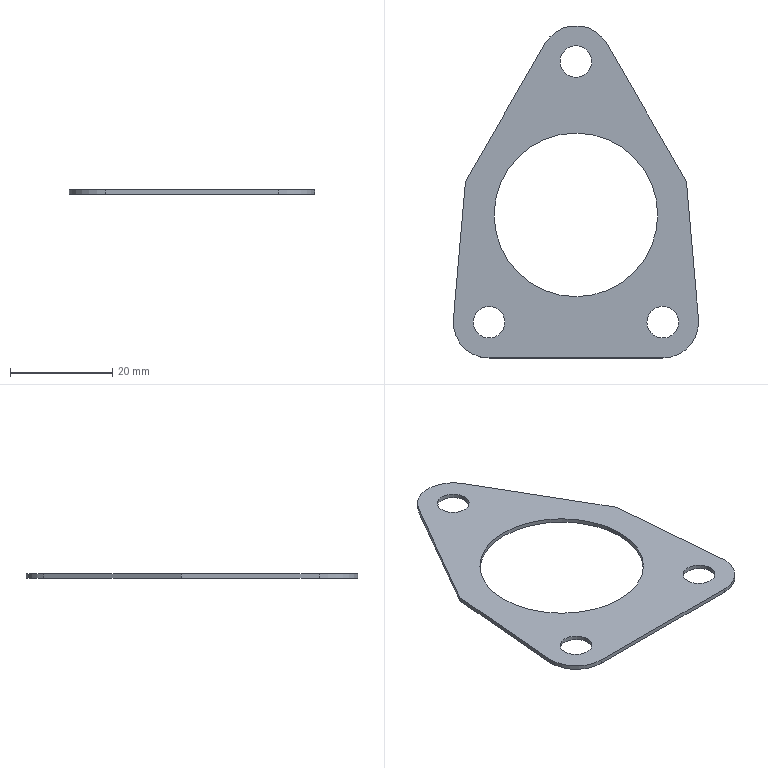Part | SolidWorks | features BaseBody 1 | 1 solid | 19 faces | box 48 x 65 x 0.8 mm | volume 1163 mm3 | cylinder 12 | plane 7 | commonest cylinder face diameters 6.2 x6 14 x4 32 x2
STEP:
#1=CARTESIAN_POINT('',(113.6,-21.,50.5));
#2=VERTEX_POINT('',#1);
#3=CARTESIAN_POINT('',(107.4,-21.,50.5));
#4=VERTEX_POINT('',#3);
#5=CARTESIAN_POINT('',(110.5,-21.,50.5));
#6=DIRECTION('',(0.,0.,-1.));
#7=DIRECTION('',(-1.,0.,0.));
#8=AXIS2_PLACEMENT_3D('',#5,#6,#7);
#9=CIRCLE('',#8,3.1);
#10=EDGE_CURVE('',#2,#4,#9,.T.);
#11=ORIENTED_EDGE('',*,*,#10,.T.);
#12=CARTESIAN_POINT('',(107.4,-21.,51.3));
#13=VERTEX_POINT('',#12);
#14=CARTESIAN_POINT('',(107.4,-21.,50.5));
#15=DIRECTION('',(0.,0.,1.));
#16=VECTOR('',#15,1000.);
#17=LINE('',#14,#16);
#18=EDGE_CURVE('',#4,#13,#17,.T.);
#19=ORIENTED_EDGE('',*,*,#18,.T.);
#20=CARTESIAN_POINT('',(113.6,-21.,51.3));
#21=VERTEX_POINT('',#20);
#22=CARTESIAN_POINT('',(110.5,-21.,51.3));
#23=DIRECTION('',(0.,0.,-1.));
#24=DIRECTION('',(-1.,0.,0.));
#25=AXIS2_PLACEMENT_3D('',#22,#23,#24);
#26=CIRCLE('',#25,3.1);
#27=EDGE_CURVE('',#21,#13,#26,.T.);
#28=ORIENTED_EDGE('',*,*,#27,.F.);
#29=CARTESIAN_POINT('',(113.6,-21.,50.5));
#30=DIRECTION('',(0.,0.,1.));
#31=VECTOR('',#30,1000.);
#32=LINE('',#29,#31);
#33=EDGE_CURVE('',#2,#21,#32,.T.);
#34=ORIENTED_EDGE('',*,*,#33,.F.);
#35=EDGE_LOOP('',(#11,#19,#28,#34));
#36=FACE_OUTER_BOUND('',#35,.T.);
#37=CARTESIAN_POINT('',(110.5,-21.,50.5));
#38=DIRECTION('',(0.,0.,1.));
#39=DIRECTION('',(1.,0.,0.));
#40=AXIS2_PLACEMENT_3D('',#37,#38,#39);
#41=CYLINDRICAL_SURFACE('',#40,3.1);
#42=ADVANCED_FACE('',(#36),#41,.F.);
#43=CARTESIAN_POINT('',(79.6,-21.,50.5));
#44=VERTEX_POINT('',#43);
#45=CARTESIAN_POINT('',(73.4,-21.,50.5));
#46=VERTEX_POINT('',#45);
#47=CARTESIAN_POINT('',(76.5,-21.,50.5));
#48=DIRECTION('',(0.,0.,-1.));
#49=DIRECTION('',(-1.,0.,0.));
#50=AXIS2_PLACEMENT_3D('',#47,#48,#49);
#51=CIRCLE('',#50,3.1);
#52=EDGE_CURVE('',#44,#46,#51,.T.);
#53=ORIENTED_EDGE('',*,*,#52,.T.);
#54=CARTESIAN_POINT('',(73.4,-21.,51.3));
#55=VERTEX_POINT('',#54);
#56=CARTESIAN_POINT('',(73.4,-21.,50.5));
#57=DIRECTION('',(0.,0.,1.));
#58=VECTOR('',#57,1000.);
#59=LINE('',#56,#58);
#60=EDGE_CURVE('',#46,#55,#59,.T.);
#61=ORIENTED_EDGE('',*,*,#60,.T.);
#62=CARTESIAN_POINT('',(79.6,-21.,51.3));
#63=VERTEX_POINT('',#62);
#64=CARTESIAN_POINT('',(76.5,-21.,51.3));
#65=DIRECTION('',(0.,0.,-1.));
#66=DIRECTION('',(-1.,0.,0.));
#67=AXIS2_PLACEMENT_3D('',#64,#65,#66);
#68=CIRCLE('',#67,3.1);
#69=EDGE_CURVE('',#63,#55,#68,.T.);
#70=ORIENTED_EDGE('',*,*,#69,.F.);
#71=CARTESIAN_POINT('',(79.6,-21.,50.5));
#72=DIRECTION('',(0.,0.,1.));
#73=VECTOR('',#72,1000.);
#74=LINE('',#71,#73);
#75=EDGE_CURVE('',#44,#63,#74,.T.);
#76=ORIENTED_EDGE('',*,*,#75,.F.);
#77=EDGE_LOOP('',(#53,#61,#70,#76));
#78=FACE_OUTER_BOUND('',#77,.T.);
#79=CARTESIAN_POINT('',(76.5,-21.,50.5));
#80=DIRECTION('',(0.,0.,1.));
#81=DIRECTION('',(1.,0.,0.));
#82=AXIS2_PLACEMENT_3D('',#79,#80,#81);
#83=CYLINDRICAL_SURFACE('',#82,3.1);
#84=ADVANCED_FACE('',(#78),#83,.F.);
#85=CARTESIAN_POINT('',(96.6,30.,50.5));
#86=VERTEX_POINT('',#85);
#87=CARTESIAN_POINT('',(90.4,30.,50.5));
#88=VERTEX_POINT('',#87);
#89=CARTESIAN_POINT('',(93.5,30.,50.5));
#90=DIRECTION('',(0.,0.,-1.));
#91=DIRECTION('',(-1.,0.,0.));
#92=AXIS2_PLACEMENT_3D('',#89,#90,#91);
#93=CIRCLE('',#92,3.1);
#94=EDGE_CURVE('',#86,#88,#93,.T.);
#95=ORIENTED_EDGE('',*,*,#94,.T.);
#96=CARTESIAN_POINT('',(90.4,30.,51.3));
#97=VERTEX_POINT('',#96);
#98=CARTESIAN_POINT('',(90.4,30.,50.5));
#99=DIRECTION('',(0.,0.,1.));
#100=VECTOR('',#99,1000.);
#101=LINE('',#98,#100);
#102=EDGE_CURVE('',#88,#97,#101,.T.);
#103=ORIENTED_EDGE('',*,*,#102,.T.);
#104=CARTESIAN_POINT('',(96.6,30.,51.3));
#105=VERTEX_POINT('',#104);
#106=CARTESIAN_POINT('',(93.5,30.,51.3));
#107=DIRECTION('',(0.,0.,-1.));
#108=DIRECTION('',(-1.,0.,0.));
#109=AXIS2_PLACEMENT_3D('',#106,#107,#108);
#110=CIRCLE('',#109,3.1);
#111=EDGE_CURVE('',#105,#97,#110,.T.);
#112=ORIENTED_EDGE('',*,*,#111,.F.);
#113=CARTESIAN_POINT('',(96.6,30.,50.5));
#114=DIRECTION('',(0.,0.,1.));
#115=VECTOR('',#114,1000.);
#116=LINE('',#113,#115);
#117=EDGE_CURVE('',#86,#105,#116,.T.);
#118=ORIENTED_EDGE('',*,*,#117,.F.);
#119=EDGE_LOOP('',(#95,#103,#112,#118));
#120=FACE_OUTER_BOUND('',#119,.T.);
#121=CARTESIAN_POINT('',(93.5,30.,50.5));
#122=DIRECTION('',(0.,0.,1.));
#123=DIRECTION('',(1.,0.,0.));
#124=AXIS2_PLACEMENT_3D('',#121,#122,#123);
#125=CYLINDRICAL_SURFACE('',#124,3.1);
#126=ADVANCED_FACE('',(#120),#125,.F.);
#127=CARTESIAN_POINT('',(109.5,0.,50.5));
#128=VERTEX_POINT('',#127);
#129=CARTESIAN_POINT('',(77.5,0.,50.5));
#130=VERTEX_POINT('',#129);
#131=CARTESIAN_POINT('',(93.5,0.,50.5));
#132=DIRECTION('',(0.,0.,-1.));
#133=DIRECTION('',(-1.,0.,0.));
#134=AXIS2_PLACEMENT_3D('',#131,#132,#133);
#135=CIRCLE('',#134,16.);
#136=EDGE_CURVE('',#128,#130,#135,.T.);
#137=ORIENTED_EDGE('',*,*,#136,.T.);
#138=CARTESIAN_POINT('',(77.5,0.,51.3));
#139=VERTEX_POINT('',#138);
#140=CARTESIAN_POINT('',(77.5,0.,50.5));
#141=DIRECTION('',(0.,0.,1.));
#142=VECTOR('',#141,1000.);
#143=LINE('',#140,#142);
#144=EDGE_CURVE('',#130,#139,#143,.T.);
#145=ORIENTED_EDGE('',*,*,#144,.T.);
#146=CARTESIAN_POINT('',(109.5,0.,51.3));
#147=VERTEX_POINT('',#146);
#148=CARTESIAN_POINT('',(93.5,0.,51.3));
#149=DIRECTION('',(0.,0.,-1.));
#150=DIRECTION('',(-1.,0.,0.));
#151=AXIS2_PLACEMENT_3D('',#148,#149,#150);
#152=CIRCLE('',#151,16.);
#153=EDGE_CURVE('',#147,#139,#152,.T.);
#154=ORIENTED_EDGE('',*,*,#153,.F.);
#155=CARTESIAN_POINT('',(109.5,0.,50.5));
#156=DIRECTION('',(0.,0.,1.));
#157=VECTOR('',#156,1000.);
#158=LINE('',#155,#157);
#159=EDGE_CURVE('',#128,#147,#158,.T.);
#160=ORIENTED_EDGE('',*,*,#159,.F.);
#161=EDGE_LOOP('',(#137,#145,#154,#160));
#162=FACE_OUTER_BOUND('',#161,.T.);
#163=CARTESIAN_POINT('',(93.5,0.,50.5));
#164=DIRECTION('',(0.,0.,1.));
#165=DIRECTION('',(1.,0.,0.));
#166=AXIS2_PLACEMENT_3D('',#163,#164,#165);
#167=CYLINDRICAL_SURFACE('',#166,16.);
#168=ADVANCED_FACE('',(#162),#167,.F.);
#169=CARTESIAN_POINT('',(117.5,-21.,50.5));
#170=VERTEX_POINT('',#169);
#171=CARTESIAN_POINT('',(110.5,-28.,50.5));
#172=VERTEX_POINT('',#171);
#173=CARTESIAN_POINT('',(110.5,-21.,50.5));
#174=DIRECTION('',(0.,0.,-1.));
#175=DIRECTION('',(-1.,0.,0.));
#176=AXIS2_PLACEMENT_3D('',#173,#174,#175);
#177=CIRCLE('',#176,7.);
#178=EDGE_CURVE('',#170,#172,#177,.T.);
#179=ORIENTED_EDGE('',*,*,#178,.F.);
#180=CARTESIAN_POINT('',(117.5,-21.,51.3));
#181=VERTEX_POINT('',#180);
#182=CARTESIAN_POINT('',(117.5,-21.,50.5));
#183=DIRECTION('',(0.,0.,1.));
#184=VECTOR('',#183,1000.);
#185=LINE('',#182,#184);
#186=EDGE_CURVE('',#170,#181,#185,.T.);
#187=ORIENTED_EDGE('',*,*,#186,.T.);
#188=CARTESIAN_POINT('',(110.5,-28.,51.3));
#189=VERTEX_POINT('',#188);
#190=CARTESIAN_POINT('',(110.5,-21.,51.3));
#191=DIRECTION('',(0.,0.,-1.));
#192=DIRECTION('',(-1.,0.,0.));
#193=AXIS2_PLACEMENT_3D('',#190,#191,#192);
#194=CIRCLE('',#193,7.);
#195=EDGE_CURVE('',#181,#189,#194,.T.);
#196=ORIENTED_EDGE('',*,*,#195,.T.);
#197=CARTESIAN_POINT('',(110.5,-28.,50.5));
#198=DIRECTION('',(0.,0.,1.));
#199=VECTOR('',#198,1000.);
#200=LINE('',#197,#199);
#201=EDGE_CURVE('',#172,#189,#200,.T.);
#202=ORIENTED_EDGE('',*,*,#201,.F.);
#203=EDGE_LOOP('',(#179,#187,#196,#202));
#204=FACE_OUTER_BOUND('',#203,.T.);
#205=CARTESIAN_POINT('',(110.5,-21.,50.5));
#206=DIRECTION('',(0.,0.,1.));
#207=DIRECTION('',(1.,0.,0.));
#208=AXIS2_PLACEMENT_3D('',#205,#206,#207);
#209=CYLINDRICAL_SURFACE('',#208,7.);
#210=ADVANCED_FACE('',(#204),#209,.T.);
#211=ORIENTED_EDGE('',*,*,#52,.F.);
#212=CARTESIAN_POINT('',(76.5,-21.,50.5));
#213=DIRECTION('',(0.,0.,-1.));
#214=DIRECTION('',(-1.,0.,0.));
#215=AXIS2_PLACEMENT_3D('',#212,#213,#214);
#216=CIRCLE('',#215,3.1);
#217=EDGE_CURVE('',#46,#44,#216,.T.);
#218=ORIENTED_EDGE('',*,*,#217,.F.);
#219=EDGE_LOOP('',(#211,#218));
#220=FACE_BOUND('',#219,.T.);
#221=ORIENTED_EDGE('',*,*,#136,.F.);
#222=CARTESIAN_POINT('',(93.5,0.,50.5));
#223=DIRECTION('',(0.,0.,-1.));
#224=DIRECTION('',(-1.,0.,0.));
#225=AXIS2_PLACEMENT_3D('',#222,#223,#224);
#226=CIRCLE('',#225,16.);
#227=EDGE_CURVE('',#130,#128,#226,.T.);
#228=ORIENTED_EDGE('',*,*,#227,.F.);
#229=EDGE_LOOP('',(#221,#228));
#230=FACE_BOUND('',#229,.T.);
#231=CARTESIAN_POINT('',(87.438,33.5,50.5));
#232=VERTEX_POINT('',#231);
#233=CARTESIAN_POINT('',(99.562,33.5,50.5));
#234=VERTEX_POINT('',#233);
#235=CARTESIAN_POINT('',(93.5,30.,50.5));
#236=DIRECTION('',(0.,0.,-1.));
#237=DIRECTION('',(-1.,0.,0.));
#238=AXIS2_PLACEMENT_3D('',#235,#236,#237);
#239=CIRCLE('',#238,7.);
#240=EDGE_CURVE('',#232,#234,#239,.T.);
#241=ORIENTED_EDGE('',*,*,#240,.T.);
#242=CARTESIAN_POINT('',(115.115,6.561,50.5));
#243=VERTEX_POINT('',#242);
#244=CARTESIAN_POINT('',(99.562,33.5,50.5));
#245=DIRECTION('',(0.5,-0.866,0.));
#246=VECTOR('',#245,1000.);
#247=LINE('',#244,#246);
#248=EDGE_CURVE('',#234,#243,#247,.T.);
#249=ORIENTED_EDGE('',*,*,#248,.T.);
#250=CARTESIAN_POINT('',(117.473,-20.39,50.5));
#251=VERTEX_POINT('',#250);
#252=CARTESIAN_POINT('',(117.473,-20.39,50.5));
#253=DIRECTION('',(0.08716,-0.9962,0.));
#254=VECTOR('',#253,1000.);
#255=LINE('',#252,#254);
#256=EDGE_CURVE('',#243,#251,#255,.T.);
#257=ORIENTED_EDGE('',*,*,#256,.T.);
#258=CARTESIAN_POINT('',(110.5,-21.,50.5));
#259=DIRECTION('',(0.,0.,-1.));
#260=DIRECTION('',(-1.,0.,0.));
#261=AXIS2_PLACEMENT_3D('',#258,#259,#260);
#262=CIRCLE('',#261,7.);
#263=EDGE_CURVE('',#251,#170,#262,.T.);
#264=ORIENTED_EDGE('',*,*,#263,.T.);
#265=ORIENTED_EDGE('',*,*,#178,.T.);
#266=CARTESIAN_POINT('',(76.5,-28.,50.5));
#267=VERTEX_POINT('',#266);
#268=CARTESIAN_POINT('',(110.5,-28.,50.5));
#269=DIRECTION('',(-1.,0.,0.));
#270=VECTOR('',#269,1000.);
#271=LINE('',#268,#270);
#272=EDGE_CURVE('',#172,#267,#271,.T.);
#273=ORIENTED_EDGE('',*,*,#272,.T.);
#274=CARTESIAN_POINT('',(69.527,-20.39,50.5));
#275=VERTEX_POINT('',#274);
#276=CARTESIAN_POINT('',(76.5,-21.,50.5));
#277=DIRECTION('',(0.,0.,-1.));
#278=DIRECTION('',(-1.,0.,0.));
#279=AXIS2_PLACEMENT_3D('',#276,#277,#278);
#280=CIRCLE('',#279,7.);
#281=EDGE_CURVE('',#267,#275,#280,.T.);
#282=ORIENTED_EDGE('',*,*,#281,.T.);
#283=CARTESIAN_POINT('',(71.885,6.561,50.5));
#284=VERTEX_POINT('',#283);
#285=CARTESIAN_POINT('',(69.527,-20.39,50.5));
#286=DIRECTION('',(0.08716,0.9962,0.));
#287=VECTOR('',#286,1000.);
#288=LINE('',#285,#287);
#289=EDGE_CURVE('',#275,#284,#288,.T.);
#290=ORIENTED_EDGE('',*,*,#289,.T.);
#291=CARTESIAN_POINT('',(87.438,33.5,50.5));
#292=DIRECTION('',(0.5,0.866,0.));
#293=VECTOR('',#292,1000.);
#294=LINE('',#291,#293);
#295=EDGE_CURVE('',#284,#232,#294,.T.);
#296=ORIENTED_EDGE('',*,*,#295,.T.);
#297=EDGE_LOOP('',(#241,#249,#257,#264,#265,#273,#282,#290,#296));
#298=FACE_OUTER_BOUND('',#297,.T.);
#299=ORIENTED_EDGE('',*,*,#94,.F.);
#300=CARTESIAN_POINT('',(93.5,30.,50.5));
#301=DIRECTION('',(0.,0.,-1.));
#302=DIRECTION('',(-1.,0.,0.));
#303=AXIS2_PLACEMENT_3D('',#300,#301,#302);
#304=CIRCLE('',#303,3.1);
#305=EDGE_CURVE('',#88,#86,#304,.T.);
#306=ORIENTED_EDGE('',*,*,#305,.F.);
#307=EDGE_LOOP('',(#299,#306));
#308=FACE_BOUND('',#307,.T.);
#309=ORIENTED_EDGE('',*,*,#10,.F.);
#310=CARTESIAN_POINT('',(110.5,-21.,50.5));
#311=DIRECTION('',(0.,0.,-1.));
#312=DIRECTION('',(-1.,0.,0.));
#313=AXIS2_PLACEMENT_3D('',#310,#311,#312);
#314=CIRCLE('',#313,3.1);
#315=EDGE_CURVE('',#4,#2,#314,.T.);
#316=ORIENTED_EDGE('',*,*,#315,.F.);
#317=EDGE_LOOP('',(#309,#316));
#318=FACE_BOUND('',#317,.T.);
#319=CARTESIAN_POINT('',(93.5,30.,50.5));
#320=DIRECTION('',(0.,0.,-1.));
#321=DIRECTION('',(-1.,0.,0.));
#322=AXIS2_PLACEMENT_3D('',#319,#320,#321);
#323=PLANE('',#322);
#324=ADVANCED_FACE('',(#220,#230,#298,#308,#318),#323,.T.);
#325=ORIENTED_EDGE('',*,*,#69,.T.);
#326=CARTESIAN_POINT('',(76.5,-21.,51.3));
#327=DIRECTION('',(0.,0.,-1.));
#328=DIRECTION('',(-1.,0.,0.));
#329=AXIS2_PLACEMENT_3D('',#326,#327,#328);
#330=CIRCLE('',#329,3.1);
#331=EDGE_CURVE('',#55,#63,#330,.T.);
#332=ORIENTED_EDGE('',*,*,#331,.T.);
#333=EDGE_LOOP('',(#325,#332));
#334=FACE_BOUND('',#333,.T.);
#335=ORIENTED_EDGE('',*,*,#153,.T.);
#336=CARTESIAN_POINT('',(93.5,0.,51.3));
#337=DIRECTION('',(0.,0.,-1.));
#338=DIRECTION('',(-1.,0.,0.));
#339=AXIS2_PLACEMENT_3D('',#336,#337,#338);
#340=CIRCLE('',#339,16.);
#341=EDGE_CURVE('',#139,#147,#340,.T.);
#342=ORIENTED_EDGE('',*,*,#341,.T.);
#343=EDGE_LOOP('',(#335,#342));
#344=FACE_BOUND('',#343,.T.);
#345=CARTESIAN_POINT('',(87.438,33.5,51.3));
#346=VERTEX_POINT('',#345);
#347=CARTESIAN_POINT('',(99.562,33.5,51.3));
#348=VERTEX_POINT('',#347);
#349=CARTESIAN_POINT('',(93.5,30.,51.3));
#350=DIRECTION('',(0.,0.,-1.));
#351=DIRECTION('',(-1.,0.,0.));
#352=AXIS2_PLACEMENT_3D('',#349,#350,#351);
#353=CIRCLE('',#352,7.);
#354=EDGE_CURVE('',#346,#348,#353,.T.);
#355=ORIENTED_EDGE('',*,*,#354,.F.);
#356=CARTESIAN_POINT('',(71.885,6.561,51.3));
#357=VERTEX_POINT('',#356);
#358=CARTESIAN_POINT('',(87.438,33.5,51.3));
#359=DIRECTION('',(0.5,0.866,0.));
#360=VECTOR('',#359,1000.);
#361=LINE('',#358,#360);
#362=EDGE_CURVE('',#357,#346,#361,.T.);
#363=ORIENTED_EDGE('',*,*,#362,.F.);
#364=CARTESIAN_POINT('',(69.527,-20.39,51.3));
#365=VERTEX_POINT('',#364);
#366=CARTESIAN_POINT('',(69.527,-20.39,51.3));
#367=DIRECTION('',(0.08716,0.9962,0.));
#368=VECTOR('',#367,1000.);
#369=LINE('',#366,#368);
#370=EDGE_CURVE('',#365,#357,#369,.T.);
#371=ORIENTED_EDGE('',*,*,#370,.F.);
#372=CARTESIAN_POINT('',(76.5,-28.,51.3));
#373=VERTEX_POINT('',#372);
#374=CARTESIAN_POINT('',(76.5,-21.,51.3));
#375=DIRECTION('',(0.,0.,-1.));
#376=DIRECTION('',(-1.,0.,0.));
#377=AXIS2_PLACEMENT_3D('',#374,#375,#376);
#378=CIRCLE('',#377,7.);
#379=EDGE_CURVE('',#373,#365,#378,.T.);
#380=ORIENTED_EDGE('',*,*,#379,.F.);
#381=CARTESIAN_POINT('',(110.5,-28.,51.3));
#382=DIRECTION('',(-1.,0.,0.));
#383=VECTOR('',#382,1000.);
#384=LINE('',#381,#383);
#385=EDGE_CURVE('',#189,#373,#384,.T.);
#386=ORIENTED_EDGE('',*,*,#385,.F.);
#387=ORIENTED_EDGE('',*,*,#195,.F.);
#388=CARTESIAN_POINT('',(117.473,-20.39,51.3));
#389=VERTEX_POINT('',#388);
#390=CARTESIAN_POINT('',(110.5,-21.,51.3));
#391=DIRECTION('',(0.,0.,-1.));
#392=DIRECTION('',(-1.,0.,0.));
#393=AXIS2_PLACEMENT_3D('',#390,#391,#392);
#394=CIRCLE('',#393,7.);
#395=EDGE_CURVE('',#389,#181,#394,.T.);
#396=ORIENTED_EDGE('',*,*,#395,.F.);
#397=CARTESIAN_POINT('',(115.115,6.561,51.3));
#398=VERTEX_POINT('',#397);
#399=CARTESIAN_POINT('',(117.473,-20.39,51.3));
#400=DIRECTION('',(0.08716,-0.9962,0.));
#401=VECTOR('',#400,1000.);
#402=LINE('',#399,#401);
#403=EDGE_CURVE('',#398,#389,#402,.T.);
#404=ORIENTED_EDGE('',*,*,#403,.F.);
#405=CARTESIAN_POINT('',(99.562,33.5,51.3));
#406=DIRECTION('',(0.5,-0.866,0.));
#407=VECTOR('',#406,1000.);
#408=LINE('',#405,#407);
#409=EDGE_CURVE('',#348,#398,#408,.T.);
#410=ORIENTED_EDGE('',*,*,#409,.F.);
#411=EDGE_LOOP('',(#355,#363,#371,#380,#386,#387,#396,#404,#410));
#412=FACE_OUTER_BOUND('',#411,.T.);
#413=ORIENTED_EDGE('',*,*,#111,.T.);
#414=CARTESIAN_POINT('',(93.5,30.,51.3));
#415=DIRECTION('',(0.,0.,-1.));
#416=DIRECTION('',(-1.,0.,0.));
#417=AXIS2_PLACEMENT_3D('',#414,#415,#416);
#418=CIRCLE('',#417,3.1);
#419=EDGE_CURVE('',#97,#105,#418,.T.);
#420=ORIENTED_EDGE('',*,*,#419,.T.);
#421=EDGE_LOOP('',(#413,#420));
#422=FACE_BOUND('',#421,.T.);
#423=ORIENTED_EDGE('',*,*,#27,.T.);
#424=CARTESIAN_POINT('',(110.5,-21.,51.3));
#425=DIRECTION('',(0.,0.,-1.));
#426=DIRECTION('',(-1.,0.,0.));
#427=AXIS2_PLACEMENT_3D('',#424,#425,#426);
#428=CIRCLE('',#427,3.1);
#429=EDGE_CURVE('',#13,#21,#428,.T.);
#430=ORIENTED_EDGE('',*,*,#429,.T.);
#431=EDGE_LOOP('',(#423,#430));
#432=FACE_BOUND('',#431,.T.);
#433=CARTESIAN_POINT('',(93.5,30.,51.3));
#434=DIRECTION('',(0.,0.,-1.));
#435=DIRECTION('',(-1.,0.,0.));
#436=AXIS2_PLACEMENT_3D('',#433,#434,#435);
#437=PLANE('',#436);
#438=ADVANCED_FACE('',(#334,#344,#412,#422,#432),#437,.F.);
#439=ORIENTED_EDGE('',*,*,#354,.T.);
#440=CARTESIAN_POINT('',(99.562,33.5,50.5));
#441=DIRECTION('',(0.,0.,1.));
#442=VECTOR('',#441,1000.);
#443=LINE('',#440,#442);
#444=EDGE_CURVE('',#234,#348,#443,.T.);
#445=ORIENTED_EDGE('',*,*,#444,.F.);
#446=ORIENTED_EDGE('',*,*,#240,.F.);
#447=CARTESIAN_POINT('',(87.438,33.5,50.5));
#448=DIRECTION('',(0.,0.,1.));
#449=VECTOR('',#448,1000.);
#450=LINE('',#447,#449);
#451=EDGE_CURVE('',#232,#346,#450,.T.);
#452=ORIENTED_EDGE('',*,*,#451,.T.);
#453=EDGE_LOOP('',(#439,#445,#446,#452));
#454=FACE_OUTER_BOUND('',#453,.T.);
#455=CARTESIAN_POINT('',(93.5,30.,50.5));
#456=DIRECTION('',(0.,0.,1.));
#457=DIRECTION('',(1.,0.,0.));
#458=AXIS2_PLACEMENT_3D('',#455,#456,#457);
#459=CYLINDRICAL_SURFACE('',#458,7.);
#460=ADVANCED_FACE('',(#454),#459,.T.);
#461=ORIENTED_EDGE('',*,*,#409,.T.);
#462=CARTESIAN_POINT('',(115.115,6.561,50.5));
#463=DIRECTION('',(0.,0.,1.));
#464=VECTOR('',#463,1000.);
#465=LINE('',#462,#464);
#466=EDGE_CURVE('',#243,#398,#465,.T.);
#467=ORIENTED_EDGE('',*,*,#466,.F.);
#468=ORIENTED_EDGE('',*,*,#248,.F.);
#469=ORIENTED_EDGE('',*,*,#444,.T.);
#470=EDGE_LOOP('',(#461,#467,#468,#469));
#471=FACE_OUTER_BOUND('',#470,.T.);
#472=CARTESIAN_POINT('',(99.562,33.5,50.5));
#473=DIRECTION('',(-0.866,-0.5,0.));
#474=DIRECTION('',(-0.5,0.866,0.));
#475=AXIS2_PLACEMENT_3D('',#472,#473,#474);
#476=PLANE('',#475);
#477=ADVANCED_FACE('',(#471),#476,.F.);
#478=ORIENTED_EDGE('',*,*,#403,.T.);
#479=CARTESIAN_POINT('',(117.473,-20.39,50.5));
#480=DIRECTION('',(0.,0.,1.));
#481=VECTOR('',#480,1000.);
#482=LINE('',#479,#481);
#483=EDGE_CURVE('',#251,#389,#482,.T.);
#484=ORIENTED_EDGE('',*,*,#483,.F.);
#485=ORIENTED_EDGE('',*,*,#256,.F.);
#486=ORIENTED_EDGE('',*,*,#466,.T.);
#487=EDGE_LOOP('',(#478,#484,#485,#486));
#488=FACE_OUTER_BOUND('',#487,.T.);
#489=CARTESIAN_POINT('',(117.473,-20.39,50.5));
#490=DIRECTION('',(-0.9962,-0.08716,0.));
#491=DIRECTION('',(-0.08716,0.9962,0.));
#492=AXIS2_PLACEMENT_3D('',#489,#490,#491);
#493=PLANE('',#492);
#494=ADVANCED_FACE('',(#488),#493,.F.);
#495=ORIENTED_EDGE('',*,*,#186,.F.);
#496=ORIENTED_EDGE('',*,*,#263,.F.);
#497=ORIENTED_EDGE('',*,*,#483,.T.);
#498=ORIENTED_EDGE('',*,*,#395,.T.);
#499=EDGE_LOOP('',(#495,#496,#497,#498));
#500=FACE_OUTER_BOUND('',#499,.T.);
#501=CARTESIAN_POINT('',(110.5,-21.,50.5));
#502=DIRECTION('',(0.,0.,1.));
#503=DIRECTION('',(1.,0.,0.));
#504=AXIS2_PLACEMENT_3D('',#501,#502,#503);
#505=CYLINDRICAL_SURFACE('',#504,7.);
#506=ADVANCED_FACE('',(#500),#505,.T.);
#507=ORIENTED_EDGE('',*,*,#385,.T.);
#508=CARTESIAN_POINT('',(76.5,-28.,50.5));
#509=DIRECTION('',(0.,0.,1.));
#510=VECTOR('',#509,1000.);
#511=LINE('',#508,#510);
#512=EDGE_CURVE('',#267,#373,#511,.T.);
#513=ORIENTED_EDGE('',*,*,#512,.F.);
#514=ORIENTED_EDGE('',*,*,#272,.F.);
#515=ORIENTED_EDGE('',*,*,#201,.T.);
#516=EDGE_LOOP('',(#507,#513,#514,#515));
#517=FACE_OUTER_BOUND('',#516,.T.);
#518=CARTESIAN_POINT('',(110.5,-28.,50.5));
#519=DIRECTION('',(0.,1.,0.));
#520=DIRECTION('',(0.,0.,-1.));
#521=AXIS2_PLACEMENT_3D('',#518,#519,#520);
#522=PLANE('',#521);
#523=ADVANCED_FACE('',(#517),#522,.F.);
#524=ORIENTED_EDGE('',*,*,#379,.T.);
#525=CARTESIAN_POINT('',(69.527,-20.39,50.5));
#526=DIRECTION('',(0.,0.,1.));
#527=VECTOR('',#526,1000.);
#528=LINE('',#525,#527);
#529=EDGE_CURVE('',#275,#365,#528,.T.);
#530=ORIENTED_EDGE('',*,*,#529,.F.);
#531=ORIENTED_EDGE('',*,*,#281,.F.);
#532=ORIENTED_EDGE('',*,*,#512,.T.);
#533=EDGE_LOOP('',(#524,#530,#531,#532));
#534=FACE_OUTER_BOUND('',#533,.T.);
#535=CARTESIAN_POINT('',(76.5,-21.,50.5));
#536=DIRECTION('',(0.,0.,1.));
#537=DIRECTION('',(1.,0.,0.));
#538=AXIS2_PLACEMENT_3D('',#535,#536,#537);
#539=CYLINDRICAL_SURFACE('',#538,7.);
#540=ADVANCED_FACE('',(#534),#539,.T.);
#541=ORIENTED_EDGE('',*,*,#370,.T.);
#542=CARTESIAN_POINT('',(71.885,6.561,50.5));
#543=DIRECTION('',(0.,0.,1.));
#544=VECTOR('',#543,1000.);
#545=LINE('',#542,#544);
#546=EDGE_CURVE('',#284,#357,#545,.T.);
#547=ORIENTED_EDGE('',*,*,#546,.F.);
#548=ORIENTED_EDGE('',*,*,#289,.F.);
#549=ORIENTED_EDGE('',*,*,#529,.T.);
#550=EDGE_LOOP('',(#541,#547,#548,#549));
#551=FACE_OUTER_BOUND('',#550,.T.);
#552=CARTESIAN_POINT('',(69.527,-20.39,50.5));
#553=DIRECTION('',(0.9962,-0.08716,0.));
#554=DIRECTION('',(-0.08716,-0.9962,0.));
#555=AXIS2_PLACEMENT_3D('',#552,#553,#554);
#556=PLANE('',#555);
#557=ADVANCED_FACE('',(#551),#556,.F.);
#558=ORIENTED_EDGE('',*,*,#362,.T.);
#559=ORIENTED_EDGE('',*,*,#451,.F.);
#560=ORIENTED_EDGE('',*,*,#295,.F.);
#561=ORIENTED_EDGE('',*,*,#546,.T.);
#562=EDGE_LOOP('',(#558,#559,#560,#561));
#563=FACE_OUTER_BOUND('',#562,.T.);
#564=CARTESIAN_POINT('',(87.438,33.5,50.5));
#565=DIRECTION('',(0.866,-0.5,0.));
#566=DIRECTION('',(-0.5,-0.866,0.));
#567=AXIS2_PLACEMENT_3D('',#564,#565,#566);
#568=PLANE('',#567);
#569=ADVANCED_FACE('',(#563),#568,.F.);
#570=ORIENTED_EDGE('',*,*,#144,.F.);
#571=ORIENTED_EDGE('',*,*,#227,.T.);
#572=ORIENTED_EDGE('',*,*,#159,.T.);
#573=ORIENTED_EDGE('',*,*,#341,.F.);
#574=EDGE_LOOP('',(#570,#571,#572,#573));
#575=FACE_OUTER_BOUND('',#574,.T.);
#576=CARTESIAN_POINT('',(93.5,0.,50.5));
#577=DIRECTION('',(0.,0.,1.));
#578=DIRECTION('',(1.,0.,0.));
#579=AXIS2_PLACEMENT_3D('',#576,#577,#578);
#580=CYLINDRICAL_SURFACE('',#579,16.);
#581=ADVANCED_FACE('',(#575),#580,.F.);
#582=ORIENTED_EDGE('',*,*,#102,.F.);
#583=ORIENTED_EDGE('',*,*,#305,.T.);
#584=ORIENTED_EDGE('',*,*,#117,.T.);
#585=ORIENTED_EDGE('',*,*,#419,.F.);
#586=EDGE_LOOP('',(#582,#583,#584,#585));
#587=FACE_OUTER_BOUND('',#586,.T.);
#588=CARTESIAN_POINT('',(93.5,30.,50.5));
#589=DIRECTION('',(0.,0.,1.));
#590=DIRECTION('',(1.,0.,0.));
#591=AXIS2_PLACEMENT_3D('',#588,#589,#590);
#592=CYLINDRICAL_SURFACE('',#591,3.1);
#593=ADVANCED_FACE('',(#587),#592,.F.);
#594=ORIENTED_EDGE('',*,*,#60,.F.);
#595=ORIENTED_EDGE('',*,*,#217,.T.);
#596=ORIENTED_EDGE('',*,*,#75,.T.);
#597=ORIENTED_EDGE('',*,*,#331,.F.);
#598=EDGE_LOOP('',(#594,#595,#596,#597));
#599=FACE_OUTER_BOUND('',#598,.T.);
#600=CARTESIAN_POINT('',(76.5,-21.,50.5));
#601=DIRECTION('',(0.,0.,1.));
#602=DIRECTION('',(1.,0.,0.));
#603=AXIS2_PLACEMENT_3D('',#600,#601,#602);
#604=CYLINDRICAL_SURFACE('',#603,3.1);
#605=ADVANCED_FACE('',(#599),#604,.F.);
#606=ORIENTED_EDGE('',*,*,#18,.F.);
#607=ORIENTED_EDGE('',*,*,#315,.T.);
#608=ORIENTED_EDGE('',*,*,#33,.T.);
#609=ORIENTED_EDGE('',*,*,#429,.F.);
#610=EDGE_LOOP('',(#606,#607,#608,#609));
#611=FACE_OUTER_BOUND('',#610,.T.);
#612=CARTESIAN_POINT('',(110.5,-21.,50.5));
#613=DIRECTION('',(0.,0.,1.));
#614=DIRECTION('',(1.,0.,0.));
#615=AXIS2_PLACEMENT_3D('',#612,#613,#614);
#616=CYLINDRICAL_SURFACE('',#615,3.1);
#617=ADVANCED_FACE('',(#611),#616,.F.);
#618=CLOSED_SHELL('',(#42,#84,#126,#168,#210,#324,#438,#460,#477,#494,#506,#523,#540,#557,#569,#581,#593,#605,#617));
#619=MANIFOLD_SOLID_BREP('',#618);
#620=CARTESIAN_POINT('',(0.,0.,0.));
#621=DIRECTION('',(0.,0.,1.));
#622=DIRECTION('',(1.,0.,0.));
#623=AXIS2_PLACEMENT_3D('',#620,#621,#622);
#624=(LENGTH_UNIT()NAMED_UNIT(*)SI_UNIT(.MILLI.,.METRE.));
#625=UNCERTAINTY_MEASURE_WITH_UNIT(LENGTH_MEASURE(0.00001),#624,'','');
#626=(NAMED_UNIT(*)PLANE_ANGLE_UNIT()SI_UNIT($,.RADIAN.));
#627=(NAMED_UNIT(*)SI_UNIT($,.STERADIAN.)SOLID_ANGLE_UNIT());
#628=(GEOMETRIC_REPRESENTATION_CONTEXT(3)GLOBAL_UNCERTAINTY_ASSIGNED_CONTEXT((#625))GLOBAL_UNIT_ASSIGNED_CONTEXT((#624,#626,#627))REPRESENTATION_CONTEXT('',''));
#629=ADVANCED_BREP_SHAPE_REPRESENTATION('',(#619,#623),#628);